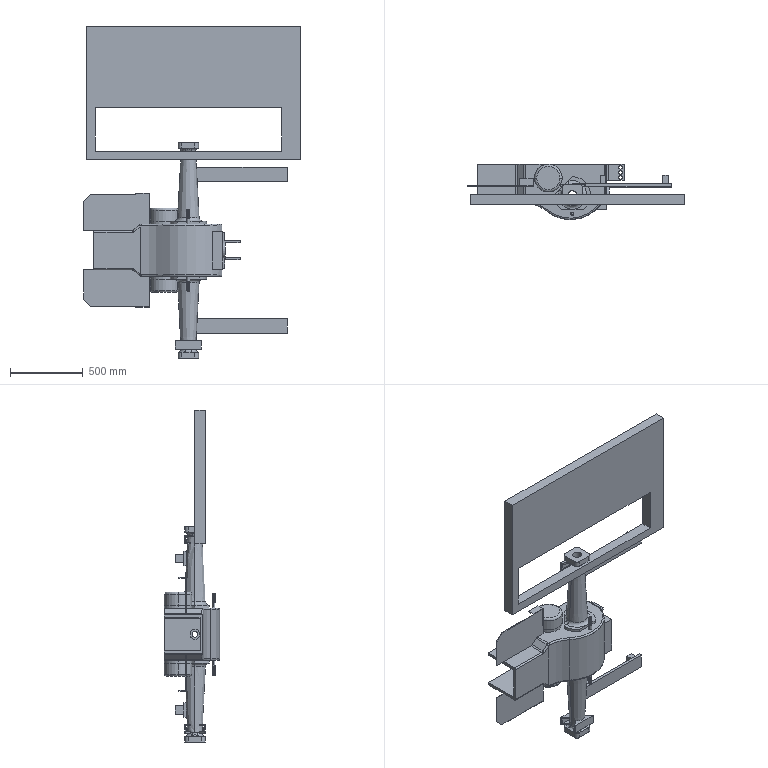Part | SolidWorks | 1 solid | 458 faces | box 1490 x 380.05 x 2280 mm | volume 110050960 mm3 | cylinder 232 | plane 168 | torus 28 | spline 22 | cone 8 | commonest cylinder face diameters 20 x170 25 x12 40 x10 5 x8 50 x8 60 x4